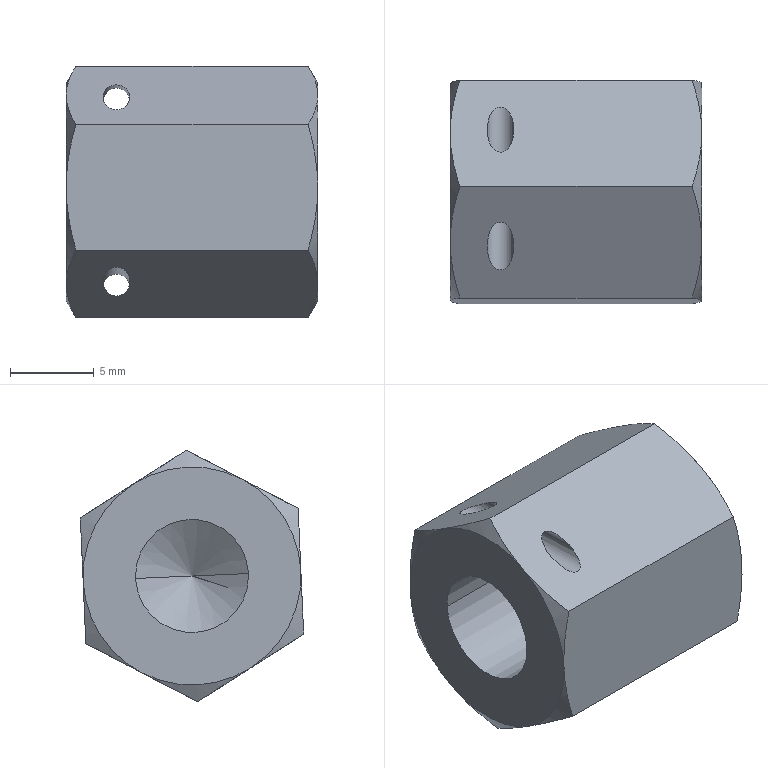Part | SolidWorks | features BaseBody 1 | 1 solid | 32 faces | box 15 x 13.316 x 14.997 mm | volume 1682 mm3 | cone 14 | plane 10 | cylinder 8 | commonest cylinder face diameters 1.6 x4 6.75 x2 8.5 x2
STEP:
#1=CARTESIAN_POINT('',(447.8,161.77,5.647));
#2=VERTEX_POINT('',#1);
#3=CARTESIAN_POINT('',(449.4,161.77,5.647));
#4=VERTEX_POINT('',#3);
#5=CARTESIAN_POINT('',(447.8,161.77,5.647));
#6=CARTESIAN_POINT('',(447.8,164.609,7.124));
#7=CARTESIAN_POINT('',(449.4,164.609,7.124));
#8=CARTESIAN_POINT('',(449.4,161.77,5.647));
#9=(BOUNDED_CURVE()B_SPLINE_CURVE(3,(#5,#6,#7,#8),.UNSPECIFIED.,.F.,.T.)B_SPLINE_CURVE_WITH_KNOTS((4,4),(4.712,7.854),.UNSPECIFIED.)CURVE()GEOMETRIC_REPRESENTATION_ITEM()RATIONAL_B_SPLINE_CURVE((1.,0.3333,0.3333,1.))REPRESENTATION_ITEM(''));
#10=EDGE_CURVE('',#2,#4,#9,.T.);
#11=ORIENTED_EDGE('',*,*,#10,.F.);
#12=CARTESIAN_POINT('',(447.8,168.711,5.343));
#13=VERTEX_POINT('',#12);
#14=CARTESIAN_POINT('',(447.8,158.747,5.779));
#15=DIRECTION('',(0.,0.999,-0.04373));
#16=VECTOR('',#15,1000.);
#17=LINE('',#14,#16);
#18=EDGE_CURVE('',#2,#13,#17,.T.);
#19=ORIENTED_EDGE('',*,*,#18,.T.);
#20=CARTESIAN_POINT('',(449.4,168.711,5.343));
#21=VERTEX_POINT('',#20);
#22=CARTESIAN_POINT('',(449.4,168.711,5.343));
#23=CARTESIAN_POINT('',(449.4,166.012,7.062));
#24=CARTESIAN_POINT('',(447.8,166.012,7.062));
#25=CARTESIAN_POINT('',(447.8,168.711,5.343));
#26=(BOUNDED_CURVE()B_SPLINE_CURVE(3,(#22,#23,#24,#25),.UNSPECIFIED.,.F.,.T.)B_SPLINE_CURVE_WITH_KNOTS((4,4),(1.571,4.712),.UNSPECIFIED.)CURVE()GEOMETRIC_REPRESENTATION_ITEM()RATIONAL_B_SPLINE_CURVE((1.,0.3333,0.3333,1.))REPRESENTATION_ITEM(''));
#27=EDGE_CURVE('',#21,#13,#26,.T.);
#28=ORIENTED_EDGE('',*,*,#27,.F.);
#29=CARTESIAN_POINT('',(449.4,158.747,5.779));
#30=DIRECTION('',(0.,0.999,-0.04373));
#31=VECTOR('',#30,1000.);
#32=LINE('',#29,#31);
#33=EDGE_CURVE('',#4,#21,#32,.T.);
#34=ORIENTED_EDGE('',*,*,#33,.F.);
#35=EDGE_LOOP('',(#11,#19,#28,#34));
#36=FACE_OUTER_BOUND('',#35,.T.);
#37=CARTESIAN_POINT('',(448.6,158.747,5.779));
#38=DIRECTION('',(0.,0.999,-0.04373));
#39=DIRECTION('',(1.,0.,0.));
#40=AXIS2_PLACEMENT_3D('',#37,#38,#39);
#41=CYLINDRICAL_SURFACE('',#40,0.8);
#42=ADVANCED_FACE('',(#36),#41,.F.);
#43=CARTESIAN_POINT('',(447.8,161.289,-5.343));
#44=VERTEX_POINT('',#43);
#45=CARTESIAN_POINT('',(449.4,161.289,-5.343));
#46=VERTEX_POINT('',#45);
#47=CARTESIAN_POINT('',(447.8,161.289,-5.343));
#48=CARTESIAN_POINT('',(447.8,158.59,-3.623));
#49=CARTESIAN_POINT('',(449.4,158.59,-3.623));
#50=CARTESIAN_POINT('',(449.4,161.289,-5.343));
#51=(BOUNDED_CURVE()B_SPLINE_CURVE(3,(#47,#48,#49,#50),.UNSPECIFIED.,.F.,.T.)B_SPLINE_CURVE_WITH_KNOTS((4,4),(1.571,4.712),.UNSPECIFIED.)CURVE()GEOMETRIC_REPRESENTATION_ITEM()RATIONAL_B_SPLINE_CURVE((1.,0.3333,0.3333,1.))REPRESENTATION_ITEM(''));
#52=EDGE_CURVE('',#44,#46,#51,.T.);
#53=ORIENTED_EDGE('',*,*,#52,.F.);
#54=CARTESIAN_POINT('',(447.8,168.23,-5.647));
#55=VERTEX_POINT('',#54);
#56=CARTESIAN_POINT('',(447.8,158.266,-5.211));
#57=DIRECTION('',(0.,0.999,-0.04373));
#58=VECTOR('',#57,1000.);
#59=LINE('',#56,#58);
#60=EDGE_CURVE('',#44,#55,#59,.T.);
#61=ORIENTED_EDGE('',*,*,#60,.T.);
#62=CARTESIAN_POINT('',(449.4,168.23,-5.647));
#63=VERTEX_POINT('',#62);
#64=CARTESIAN_POINT('',(449.4,168.23,-5.647));
#65=CARTESIAN_POINT('',(449.4,171.068,-4.169));
#66=CARTESIAN_POINT('',(447.8,171.068,-4.169));
#67=CARTESIAN_POINT('',(447.8,168.23,-5.647));
#68=(BOUNDED_CURVE()B_SPLINE_CURVE(3,(#64,#65,#66,#67),.UNSPECIFIED.,.F.,.T.)B_SPLINE_CURVE_WITH_KNOTS((4,4),(4.712,7.854),.UNSPECIFIED.)CURVE()GEOMETRIC_REPRESENTATION_ITEM()RATIONAL_B_SPLINE_CURVE((1.,0.3333,0.3333,1.))REPRESENTATION_ITEM(''));
#69=EDGE_CURVE('',#63,#55,#68,.T.);
#70=ORIENTED_EDGE('',*,*,#69,.F.);
#71=CARTESIAN_POINT('',(449.4,158.266,-5.211));
#72=DIRECTION('',(0.,0.999,-0.04373));
#73=VECTOR('',#72,1000.);
#74=LINE('',#71,#73);
#75=EDGE_CURVE('',#46,#63,#74,.T.);
#76=ORIENTED_EDGE('',*,*,#75,.F.);
#77=EDGE_LOOP('',(#53,#61,#70,#76));
#78=FACE_OUTER_BOUND('',#77,.T.);
#79=CARTESIAN_POINT('',(448.6,158.266,-5.211));
#80=DIRECTION('',(0.,0.999,-0.04373));
#81=DIRECTION('',(1.,0.,0.));
#82=AXIS2_PLACEMENT_3D('',#79,#80,#81);
#83=CYLINDRICAL_SURFACE('',#82,0.8);
#84=ADVANCED_FACE('',(#78),#83,.F.);
#85=CARTESIAN_POINT('',(458.628,165.,0.));
#86=VERTEX_POINT('',#85);
#87=CARTESIAN_POINT('',(456.6,168.372,-0.1476));
#88=VERTEX_POINT('',#87);
#89=CARTESIAN_POINT('',(456.6,168.372,-0.1476));
#90=DIRECTION('',(-0.515,0.8563,-0.03748));
#91=VECTOR('',#90,1000.);
#92=LINE('',#89,#91);
#93=EDGE_CURVE('',#86,#88,#92,.T.);
#94=ORIENTED_EDGE('',*,*,#93,.F.);
#95=CARTESIAN_POINT('',(456.6,161.628,0.1476));
#96=VERTEX_POINT('',#95);
#97=CARTESIAN_POINT('',(456.6,161.628,0.1476));
#98=DIRECTION('',(-0.515,-0.8563,0.03748));
#99=VECTOR('',#98,1000.);
#100=LINE('',#97,#99);
#101=EDGE_CURVE('',#86,#96,#100,.T.);
#102=ORIENTED_EDGE('',*,*,#101,.T.);
#103=CARTESIAN_POINT('',(456.6,165.,0.));
#104=DIRECTION('',(1.,0.,0.));
#105=DIRECTION('',(0.,0.999,-0.04373));
#106=AXIS2_PLACEMENT_3D('',#103,#104,#105);
#107=CIRCLE('',#106,3.375);
#108=EDGE_CURVE('',#88,#96,#107,.T.);
#109=ORIENTED_EDGE('',*,*,#108,.F.);
#110=EDGE_LOOP('',(#94,#102,#109));
#111=FACE_OUTER_BOUND('',#110,.T.);
#112=CARTESIAN_POINT('',(456.6,165.,0.));
#113=DIRECTION('',(-1.,0.,0.));
#114=DIRECTION('',(0.,0.999,-0.04373));
#115=AXIS2_PLACEMENT_3D('',#112,#113,#114);
#116=CONICAL_SURFACE('',#115,3.375,1.03);
#117=ADVANCED_FACE('',(#111),#116,.F.);
#118=CARTESIAN_POINT('',(456.6,160.754,0.1858));
#119=VERTEX_POINT('',#118);
#120=CARTESIAN_POINT('',(456.6,169.246,-0.1858));
#121=VERTEX_POINT('',#120);
#122=CARTESIAN_POINT('',(456.6,165.,0.));
#123=DIRECTION('',(-1.,0.,0.));
#124=DIRECTION('',(0.,0.999,-0.04373));
#125=AXIS2_PLACEMENT_3D('',#122,#123,#124);
#126=CIRCLE('',#125,4.25);
#127=EDGE_CURVE('',#119,#121,#126,.T.);
#128=ORIENTED_EDGE('',*,*,#127,.F.);
#129=CARTESIAN_POINT('',(453.6,160.754,0.1858));
#130=VERTEX_POINT('',#129);
#131=CARTESIAN_POINT('',(456.6,160.754,0.1858));
#132=DIRECTION('',(-1.,0.,0.));
#133=VECTOR('',#132,1000.);
#134=LINE('',#131,#133);
#135=EDGE_CURVE('',#119,#130,#134,.T.);
#136=ORIENTED_EDGE('',*,*,#135,.T.);
#137=CARTESIAN_POINT('',(453.6,169.246,-0.1858));
#138=VERTEX_POINT('',#137);
#139=CARTESIAN_POINT('',(453.6,165.,0.));
#140=DIRECTION('',(-1.,0.,0.));
#141=DIRECTION('',(0.,0.999,-0.04373));
#142=AXIS2_PLACEMENT_3D('',#139,#140,#141);
#143=CIRCLE('',#142,4.25);
#144=EDGE_CURVE('',#130,#138,#143,.T.);
#145=ORIENTED_EDGE('',*,*,#144,.T.);
#146=CARTESIAN_POINT('',(456.6,169.246,-0.1858));
#147=DIRECTION('',(-1.,0.,0.));
#148=VECTOR('',#147,1000.);
#149=LINE('',#146,#148);
#150=EDGE_CURVE('',#121,#138,#149,.T.);
#151=ORIENTED_EDGE('',*,*,#150,.F.);
#152=EDGE_LOOP('',(#128,#136,#145,#151));
#153=FACE_OUTER_BOUND('',#152,.T.);
#154=CARTESIAN_POINT('',(456.6,165.,0.));
#155=DIRECTION('',(-1.,0.,0.));
#156=DIRECTION('',(0.,0.999,-0.04373));
#157=AXIS2_PLACEMENT_3D('',#154,#155,#156);
#158=CYLINDRICAL_SURFACE('',#157,4.25);
#159=ADVANCED_FACE('',(#153),#158,.F.);
#160=CARTESIAN_POINT('',(453.6,168.372,-0.1476));
#161=VERTEX_POINT('',#160);
#162=CARTESIAN_POINT('',(453.6,161.628,0.1476));
#163=VERTEX_POINT('',#162);
#164=CARTESIAN_POINT('',(453.6,165.,0.));
#165=DIRECTION('',(1.,0.,0.));
#166=DIRECTION('',(0.,0.999,-0.04373));
#167=AXIS2_PLACEMENT_3D('',#164,#165,#166);
#168=CIRCLE('',#167,3.375);
#169=EDGE_CURVE('',#161,#163,#168,.T.);
#170=ORIENTED_EDGE('',*,*,#169,.T.);
#171=CARTESIAN_POINT('',(445.6,161.628,0.1476));
#172=VERTEX_POINT('',#171);
#173=CARTESIAN_POINT('',(456.6,161.628,0.1476));
#174=DIRECTION('',(-1.,0.,0.));
#175=VECTOR('',#174,1000.);
#176=LINE('',#173,#175);
#177=EDGE_CURVE('',#163,#172,#176,.T.);
#178=ORIENTED_EDGE('',*,*,#177,.T.);
#179=CARTESIAN_POINT('',(445.6,168.372,-0.1476));
#180=VERTEX_POINT('',#179);
#181=CARTESIAN_POINT('',(445.6,165.,0.));
#182=DIRECTION('',(-1.,0.,0.));
#183=DIRECTION('',(0.,0.999,-0.04373));
#184=AXIS2_PLACEMENT_3D('',#181,#182,#183);
#185=CIRCLE('',#184,3.375);
#186=EDGE_CURVE('',#172,#180,#185,.T.);
#187=ORIENTED_EDGE('',*,*,#186,.T.);
#188=CARTESIAN_POINT('',(456.6,168.372,-0.1476));
#189=DIRECTION('',(-1.,0.,0.));
#190=VECTOR('',#189,1000.);
#191=LINE('',#188,#190);
#192=EDGE_CURVE('',#161,#180,#191,.T.);
#193=ORIENTED_EDGE('',*,*,#192,.F.);
#194=EDGE_LOOP('',(#170,#178,#187,#193));
#195=FACE_OUTER_BOUND('',#194,.T.);
#196=CARTESIAN_POINT('',(456.6,165.,0.));
#197=DIRECTION('',(-1.,0.,0.));
#198=DIRECTION('',(0.,0.999,-0.04373));
#199=AXIS2_PLACEMENT_3D('',#196,#197,#198);
#200=CYLINDRICAL_SURFACE('',#199,3.375);
#201=ADVANCED_FACE('',(#195),#200,.F.);
#202=ORIENTED_EDGE('',*,*,#69,.T.);
#203=CARTESIAN_POINT('',(447.8,168.23,-5.647));
#204=CARTESIAN_POINT('',(447.8,165.391,-7.124));
#205=CARTESIAN_POINT('',(449.4,165.391,-7.124));
#206=CARTESIAN_POINT('',(449.4,168.23,-5.647));
#207=(BOUNDED_CURVE()B_SPLINE_CURVE(3,(#203,#204,#205,#206),.UNSPECIFIED.,.F.,.T.)B_SPLINE_CURVE_WITH_KNOTS((4,4),(1.571,4.712),.UNSPECIFIED.)CURVE()GEOMETRIC_REPRESENTATION_ITEM()RATIONAL_B_SPLINE_CURVE((1.,0.3333,0.3333,1.))REPRESENTATION_ITEM(''));
#208=EDGE_CURVE('',#55,#63,#207,.T.);
#209=ORIENTED_EDGE('',*,*,#208,.T.);
#210=EDGE_LOOP('',(#202,#209));
#211=FACE_BOUND('',#210,.T.);
#212=CARTESIAN_POINT('',(460.019,164.672,-7.498));
#213=VERTEX_POINT('',#212);
#214=CARTESIAN_POINT('',(460.6,168.001,-5.766));
#215=VERTEX_POINT('',#214);
#216=CARTESIAN_POINT('',(460.019,164.672,-7.498));
#217=CARTESIAN_POINT('',(460.197,165.216,-7.215));
#218=CARTESIAN_POINT('',(460.343,165.765,-6.929));
#219=CARTESIAN_POINT('',(460.545,166.873,-6.353));
#220=CARTESIAN_POINT('',(460.6,167.434,-6.061));
#221=CARTESIAN_POINT('',(460.6,168.001,-5.766));
#222=B_SPLINE_CURVE_WITH_KNOTS('',3,(#216,#217,#218,#219,#220,#221),.UNSPECIFIED.,.F.,.F.,(4,2,4),(0.000000238,0.001899,0.003797),.UNSPECIFIED.);
#223=EDGE_CURVE('',#213,#215,#222,.T.);
#224=ORIENTED_EDGE('',*,*,#223,.F.);
#225=CARTESIAN_POINT('',(446.181,164.672,-7.498));
#226=VERTEX_POINT('',#225);
#227=CARTESIAN_POINT('',(445.6,164.672,-7.498));
#228=DIRECTION('',(1.,0.,0.));
#229=VECTOR('',#228,1000.);
#230=LINE('',#227,#229);
#231=EDGE_CURVE('',#226,#213,#230,.T.);
#232=ORIENTED_EDGE('',*,*,#231,.F.);
#233=CARTESIAN_POINT('',(445.6,168.001,-5.766));
#234=VERTEX_POINT('',#233);
#235=CARTESIAN_POINT('',(445.6,168.001,-5.766));
#236=CARTESIAN_POINT('',(445.6,167.718,-5.913));
#237=CARTESIAN_POINT('',(445.614,167.434,-6.061));
#238=CARTESIAN_POINT('',(445.667,166.873,-6.353));
#239=CARTESIAN_POINT('',(445.706,166.594,-6.498));
#240=CARTESIAN_POINT('',(445.858,165.763,-6.931));
#241=CARTESIAN_POINT('',(446.004,165.215,-7.216));
#242=CARTESIAN_POINT('',(446.181,164.672,-7.498));
#243=B_SPLINE_CURVE_WITH_KNOTS('',3,(#235,#236,#237,#238,#239,#240,#241,#242),.UNSPECIFIED.,.F.,.F.,(4,2,2,4),(0.003797,0.004743,0.005689,0.00758),.UNSPECIFIED.);
#244=EDGE_CURVE('',#234,#226,#243,.T.);
#245=ORIENTED_EDGE('',*,*,#244,.F.);
#246=CARTESIAN_POINT('',(446.181,171.33,-4.033));
#247=VERTEX_POINT('',#246);
#248=CARTESIAN_POINT('',(446.181,171.33,-4.033));
#249=CARTESIAN_POINT('',(446.003,170.785,-4.317));
#250=CARTESIAN_POINT('',(445.857,170.237,-4.602));
#251=CARTESIAN_POINT('',(445.655,169.128,-5.179));
#252=CARTESIAN_POINT('',(445.6,168.568,-5.471));
#253=CARTESIAN_POINT('',(445.6,168.001,-5.766));
#254=B_SPLINE_CURVE_WITH_KNOTS('',3,(#248,#249,#250,#251,#252,#253),.UNSPECIFIED.,.F.,.F.,(4,2,4),(0.000000238,0.001899,0.003797),.UNSPECIFIED.);
#255=EDGE_CURVE('',#247,#234,#254,.T.);
#256=ORIENTED_EDGE('',*,*,#255,.F.);
#257=CARTESIAN_POINT('',(460.019,171.33,-4.033));
#258=VERTEX_POINT('',#257);
#259=CARTESIAN_POINT('',(445.6,171.33,-4.033));
#260=DIRECTION('',(1.,0.,0.));
#261=VECTOR('',#260,1000.);
#262=LINE('',#259,#261);
#263=EDGE_CURVE('',#247,#258,#262,.T.);
#264=ORIENTED_EDGE('',*,*,#263,.T.);
#265=CARTESIAN_POINT('',(460.6,168.001,-5.766));
#266=CARTESIAN_POINT('',(460.6,168.283,-5.619));
#267=CARTESIAN_POINT('',(460.586,168.567,-5.471));
#268=CARTESIAN_POINT('',(460.533,169.128,-5.179));
#269=CARTESIAN_POINT('',(460.494,169.407,-5.034));
#270=CARTESIAN_POINT('',(460.342,170.239,-4.601));
#271=CARTESIAN_POINT('',(460.196,170.786,-4.316));
#272=CARTESIAN_POINT('',(460.019,171.33,-4.033));
#273=B_SPLINE_CURVE_WITH_KNOTS('',3,(#265,#266,#267,#268,#269,#270,#271,#272),.UNSPECIFIED.,.F.,.F.,(4,2,2,4),(0.003797,0.004743,0.005689,0.00758),.UNSPECIFIED.);
#274=EDGE_CURVE('',#215,#258,#273,.T.);
#275=ORIENTED_EDGE('',*,*,#274,.F.);
#276=EDGE_LOOP('',(#224,#232,#245,#256,#264,#275));
#277=FACE_OUTER_BOUND('',#276,.T.);
#278=CARTESIAN_POINT('',(445.6,171.33,-4.033));
#279=DIRECTION('',(0.,-0.4617,0.8871));
#280=DIRECTION('',(0.,0.8871,0.4617));
#281=AXIS2_PLACEMENT_3D('',#278,#279,#280);
#282=PLANE('',#281);
#283=ADVANCED_FACE('',(#211,#277),#282,.F.);
#284=CARTESIAN_POINT('',(449.4,161.289,-5.343));
#285=CARTESIAN_POINT('',(449.4,163.988,-7.062));
#286=CARTESIAN_POINT('',(447.8,163.988,-7.062));
#287=CARTESIAN_POINT('',(447.8,161.289,-5.343));
#288=(BOUNDED_CURVE()B_SPLINE_CURVE(3,(#284,#285,#286,#287),.UNSPECIFIED.,.F.,.T.)B_SPLINE_CURVE_WITH_KNOTS((4,4),(4.712,7.854),.UNSPECIFIED.)CURVE()GEOMETRIC_REPRESENTATION_ITEM()RATIONAL_B_SPLINE_CURVE((1.,0.3333,0.3333,1.))REPRESENTATION_ITEM(''));
#289=EDGE_CURVE('',#46,#44,#288,.T.);
#290=ORIENTED_EDGE('',*,*,#289,.T.);
#291=ORIENTED_EDGE('',*,*,#52,.T.);
#292=EDGE_LOOP('',(#290,#291));
#293=FACE_BOUND('',#292,.T.);
#294=CARTESIAN_POINT('',(460.019,158.342,-3.465));
#295=VERTEX_POINT('',#294);
#296=CARTESIAN_POINT('',(460.6,161.507,-5.482));
#297=VERTEX_POINT('',#296);
#298=CARTESIAN_POINT('',(460.019,158.342,-3.465));
#299=CARTESIAN_POINT('',(460.197,158.86,-3.795));
#300=CARTESIAN_POINT('',(460.343,159.381,-4.127));
#301=CARTESIAN_POINT('',(460.545,160.435,-4.799));
#302=CARTESIAN_POINT('',(460.6,160.968,-5.138));
#303=CARTESIAN_POINT('',(460.6,161.507,-5.482));
#304=B_SPLINE_CURVE_WITH_KNOTS('',3,(#298,#299,#300,#301,#302,#303),.UNSPECIFIED.,.F.,.F.,(4,2,4),(0.000000238,0.001899,0.003797),.UNSPECIFIED.);
#305=EDGE_CURVE('',#295,#297,#304,.T.);
#306=ORIENTED_EDGE('',*,*,#305,.F.);
#307=CARTESIAN_POINT('',(446.181,158.342,-3.465));
#308=VERTEX_POINT('',#307);
#309=CARTESIAN_POINT('',(445.6,158.342,-3.465));
#310=DIRECTION('',(1.,0.,0.));
#311=VECTOR('',#310,1000.);
#312=LINE('',#309,#311);
#313=EDGE_CURVE('',#308,#295,#312,.T.);
#314=ORIENTED_EDGE('',*,*,#313,.F.);
#315=CARTESIAN_POINT('',(445.6,161.507,-5.482));
#316=VERTEX_POINT('',#315);
#317=CARTESIAN_POINT('',(445.6,161.507,-5.482));
#318=CARTESIAN_POINT('',(445.6,161.238,-5.311));
#319=CARTESIAN_POINT('',(445.614,160.969,-5.139));
#320=CARTESIAN_POINT('',(445.667,160.435,-4.799));
#321=CARTESIAN_POINT('',(445.706,160.17,-4.63));
#322=CARTESIAN_POINT('',(445.858,159.379,-4.126));
#323=CARTESIAN_POINT('',(446.004,158.859,-3.794));
#324=CARTESIAN_POINT('',(446.181,158.342,-3.465));
#325=B_SPLINE_CURVE_WITH_KNOTS('',3,(#317,#318,#319,#320,#321,#322,#323,#324),.UNSPECIFIED.,.F.,.F.,(4,2,2,4),(0.003797,0.004743,0.005689,0.00758),.UNSPECIFIED.);
#326=EDGE_CURVE('',#316,#308,#325,.T.);
#327=ORIENTED_EDGE('',*,*,#326,.F.);
#328=CARTESIAN_POINT('',(446.181,164.672,-7.498));
#329=CARTESIAN_POINT('',(446.003,164.154,-7.168));
#330=CARTESIAN_POINT('',(445.857,163.633,-6.836));
#331=CARTESIAN_POINT('',(445.655,162.579,-6.165));
#332=CARTESIAN_POINT('',(445.6,162.046,-5.825));
#333=CARTESIAN_POINT('',(445.6,161.507,-5.482));
#334=B_SPLINE_CURVE_WITH_KNOTS('',3,(#328,#329,#330,#331,#332,#333),.UNSPECIFIED.,.F.,.F.,(4,2,4),(0.000000238,0.001899,0.003797),.UNSPECIFIED.);
#335=EDGE_CURVE('',#226,#316,#334,.T.);
#336=ORIENTED_EDGE('',*,*,#335,.F.);
#337=ORIENTED_EDGE('',*,*,#231,.T.);
#338=CARTESIAN_POINT('',(460.6,161.507,-5.482));
#339=CARTESIAN_POINT('',(460.6,161.776,-5.653));
#340=CARTESIAN_POINT('',(460.586,162.045,-5.825));
#341=CARTESIAN_POINT('',(460.533,162.579,-6.165));
#342=CARTESIAN_POINT('',(460.494,162.844,-6.334));
#343=CARTESIAN_POINT('',(460.342,163.635,-6.837));
#344=CARTESIAN_POINT('',(460.196,164.155,-7.169));
#345=CARTESIAN_POINT('',(460.019,164.672,-7.498));
#346=B_SPLINE_CURVE_WITH_KNOTS('',3,(#338,#339,#340,#341,#342,#343,#344,#345),.UNSPECIFIED.,.F.,.F.,(4,2,2,4),(0.003797,0.004743,0.005689,0.00758),.UNSPECIFIED.);
#347=EDGE_CURVE('',#297,#213,#346,.T.);
#348=ORIENTED_EDGE('',*,*,#347,.F.);
#349=EDGE_LOOP('',(#306,#314,#327,#336,#337,#348));
#350=FACE_OUTER_BOUND('',#349,.T.);
#351=CARTESIAN_POINT('',(445.6,164.672,-7.498));
#352=DIRECTION('',(0.,0.5374,0.8433));
#353=DIRECTION('',(0.,0.8433,-0.5374));
#354=AXIS2_PLACEMENT_3D('',#351,#352,#353);
#355=PLANE('',#354);
#356=ADVANCED_FACE('',(#293,#350),#355,.F.);
#357=CARTESIAN_POINT('',(460.019,158.67,4.033));
#358=VERTEX_POINT('',#357);
#359=CARTESIAN_POINT('',(460.6,158.506,0.2842));
#360=VERTEX_POINT('',#359);
#361=CARTESIAN_POINT('',(460.019,158.67,4.033));
#362=CARTESIAN_POINT('',(460.196,158.644,3.423));
#363=CARTESIAN_POINT('',(460.343,158.616,2.799));
#364=CARTESIAN_POINT('',(460.545,158.562,1.548));
#365=CARTESIAN_POINT('',(460.6,158.534,0.9189));
#366=CARTESIAN_POINT('',(460.6,158.506,0.2842));
#367=B_SPLINE_CURVE_WITH_KNOTS('',3,(#361,#362,#363,#364,#365,#366),.UNSPECIFIED.,.F.,.F.,(4,2,4),(0.007076,0.008976,0.01088),.UNSPECIFIED.);
#368=EDGE_CURVE('',#358,#360,#367,.T.);
#369=ORIENTED_EDGE('',*,*,#368,.F.);
#370=CARTESIAN_POINT('',(446.181,158.67,4.033));
#371=VERTEX_POINT('',#370);
#372=CARTESIAN_POINT('',(445.6,158.67,4.033));
#373=DIRECTION('',(1.,0.,0.));
#374=VECTOR('',#373,1000.);
#375=LINE('',#372,#374);
#376=EDGE_CURVE('',#371,#358,#375,.T.);
#377=ORIENTED_EDGE('',*,*,#376,.F.);
#378=CARTESIAN_POINT('',(445.6,158.506,0.2842));
#379=VERTEX_POINT('',#378);
#380=CARTESIAN_POINT('',(445.6,158.506,0.2842));
#381=CARTESIAN_POINT('',(445.6,158.534,0.9189));
#382=CARTESIAN_POINT('',(445.655,158.562,1.548));
#383=CARTESIAN_POINT('',(445.857,158.616,2.799));
#384=CARTESIAN_POINT('',(446.004,158.644,3.423));
#385=CARTESIAN_POINT('',(446.181,158.67,4.033));
#386=B_SPLINE_CURVE_WITH_KNOTS('',3,(#380,#381,#382,#383,#384,#385),.UNSPECIFIED.,.F.,.F.,(4,2,4),(0.02975,0.03165,0.03354),.UNSPECIFIED.);
#387=EDGE_CURVE('',#379,#371,#386,.T.);
#388=ORIENTED_EDGE('',*,*,#387,.F.);
#389=CARTESIAN_POINT('',(446.181,158.342,-3.465));
#390=CARTESIAN_POINT('',(446.005,158.369,-2.858));
#391=CARTESIAN_POINT('',(445.86,158.396,-2.244));
#392=CARTESIAN_POINT('',(445.707,158.437,-1.306));
#393=CARTESIAN_POINT('',(445.667,158.45,-0.991));
#394=CARTESIAN_POINT('',(445.614,158.478,-0.3534));
#395=CARTESIAN_POINT('',(445.6,158.492,-0.03342));
#396=CARTESIAN_POINT('',(445.6,158.506,0.2842));
#397=B_SPLINE_CURVE_WITH_KNOTS('',3,(#389,#390,#391,#392,#393,#394,#395,#396),.UNSPECIFIED.,.F.,.F.,(4,2,2,4),(0.02595,0.02785,0.0288,0.02975),.UNSPECIFIED.);
#398=EDGE_CURVE('',#308,#379,#397,.T.);
#399=ORIENTED_EDGE('',*,*,#398,.F.);
#400=ORIENTED_EDGE('',*,*,#313,.T.);
#401=CARTESIAN_POINT('',(460.6,158.506,0.2842));
#402=CARTESIAN_POINT('',(460.6,158.492,-0.03342));
#403=CARTESIAN_POINT('',(460.586,158.478,-0.3534));
#404=CARTESIAN_POINT('',(460.533,158.45,-0.991));
#405=CARTESIAN_POINT('',(460.493,158.437,-1.306));
#406=CARTESIAN_POINT('',(460.34,158.396,-2.244));
#407=CARTESIAN_POINT('',(460.195,158.369,-2.858));
#408=CARTESIAN_POINT('',(460.019,158.342,-3.465));
#409=B_SPLINE_CURVE_WITH_KNOTS('',3,(#401,#402,#403,#404,#405,#406,#407,#408),.UNSPECIFIED.,.F.,.F.,(4,2,2,4),(0.01088,0.01183,0.01278,0.01468),.UNSPECIFIED.);
#410=EDGE_CURVE('',#360,#295,#409,.T.);
#411=ORIENTED_EDGE('',*,*,#410,.F.);
#412=EDGE_LOOP('',(#369,#377,#388,#399,#400,#411));
#413=FACE_OUTER_BOUND('',#412,.T.);
#414=CARTESIAN_POINT('',(445.6,158.342,-3.465));
#415=DIRECTION('',(0.,0.999,-0.04373));
#416=DIRECTION('',(0.,-0.04373,-0.999));
#417=AXIS2_PLACEMENT_3D('',#414,#415,#416);
#418=PLANE('',#417);
#419=ADVANCED_FACE('',(#413),#418,.F.);
#420=CARTESIAN_POINT('',(449.4,161.77,5.647));
#421=CARTESIAN_POINT('',(449.4,158.932,4.169));
#422=CARTESIAN_POINT('',(447.8,158.932,4.169));
#423=CARTESIAN_POINT('',(447.8,161.77,5.647));
#424=(BOUNDED_CURVE()B_SPLINE_CURVE(3,(#420,#421,#422,#423),.UNSPECIFIED.,.F.,.T.)B_SPLINE_CURVE_WITH_KNOTS((4,4),(1.571,4.712),.UNSPECIFIED.)CURVE()GEOMETRIC_REPRESENTATION_ITEM()RATIONAL_B_SPLINE_CURVE((1.,0.3333,0.3333,1.))REPRESENTATION_ITEM(''));
#425=EDGE_CURVE('',#4,#2,#424,.T.);
#426=ORIENTED_EDGE('',*,*,#425,.T.);
#427=ORIENTED_EDGE('',*,*,#10,.T.);
#428=EDGE_LOOP('',(#426,#427));
#429=FACE_BOUND('',#428,.T.);
#430=CARTESIAN_POINT('',(460.019,165.328,7.498));
#431=VERTEX_POINT('',#430);
#432=CARTESIAN_POINT('',(460.6,161.999,5.766));
#433=VERTEX_POINT('',#432);
#434=CARTESIAN_POINT('',(460.019,165.328,7.498));
#435=CARTESIAN_POINT('',(460.197,164.784,7.215));
#436=CARTESIAN_POINT('',(460.343,164.235,6.929));
#437=CARTESIAN_POINT('',(460.545,163.127,6.353));
#438=CARTESIAN_POINT('',(460.6,162.566,6.061));
#439=CARTESIAN_POINT('',(460.6,161.999,5.766));
#440=B_SPLINE_CURVE_WITH_KNOTS('',3,(#434,#435,#436,#437,#438,#439),.UNSPECIFIED.,.F.,.F.,(4,2,4),(0.000000238,0.001899,0.003797),.UNSPECIFIED.);
#441=EDGE_CURVE('',#431,#433,#440,.T.);
#442=ORIENTED_EDGE('',*,*,#441,.F.);
#443=CARTESIAN_POINT('',(446.181,165.328,7.498));
#444=VERTEX_POINT('',#443);
#445=CARTESIAN_POINT('',(445.6,165.328,7.498));
#446=DIRECTION('',(1.,0.,0.));
#447=VECTOR('',#446,1000.);
#448=LINE('',#445,#447);
#449=EDGE_CURVE('',#444,#431,#448,.T.);
#450=ORIENTED_EDGE('',*,*,#449,.F.);
#451=CARTESIAN_POINT('',(445.6,161.999,5.766));
#452=VERTEX_POINT('',#451);
#453=CARTESIAN_POINT('',(445.6,161.999,5.766));
#454=CARTESIAN_POINT('',(445.6,162.282,5.913));
#455=CARTESIAN_POINT('',(445.614,162.566,6.061));
#456=CARTESIAN_POINT('',(445.667,163.127,6.353));
#457=CARTESIAN_POINT('',(445.706,163.406,6.498));
#458=CARTESIAN_POINT('',(445.858,164.237,6.931));
#459=CARTESIAN_POINT('',(446.004,164.785,7.216));
#460=CARTESIAN_POINT('',(446.181,165.328,7.498));
#461=B_SPLINE_CURVE_WITH_KNOTS('',3,(#453,#454,#455,#456,#457,#458,#459,#460),.UNSPECIFIED.,.F.,.F.,(4,2,2,4),(0.003797,0.004743,0.005689,0.00758),.UNSPECIFIED.);
#462=EDGE_CURVE('',#452,#444,#461,.T.);
#463=ORIENTED_EDGE('',*,*,#462,.F.);
#464=CARTESIAN_POINT('',(446.181,158.67,4.033));
#465=CARTESIAN_POINT('',(446.003,159.215,4.317));
#466=CARTESIAN_POINT('',(445.857,159.763,4.602));
#467=CARTESIAN_POINT('',(445.655,160.872,5.179));
#468=CARTESIAN_POINT('',(445.6,161.432,5.471));
#469=CARTESIAN_POINT('',(445.6,161.999,5.766));
#470=B_SPLINE_CURVE_WITH_KNOTS('',3,(#464,#465,#466,#467,#468,#469),.UNSPECIFIED.,.F.,.F.,(4,2,4),(0.000000238,0.001899,0.003797),.UNSPECIFIED.);
#471=EDGE_CURVE('',#371,#452,#470,.T.);
#472=ORIENTED_EDGE('',*,*,#471,.F.);
#473=ORIENTED_EDGE('',*,*,#376,.T.);
#474=CARTESIAN_POINT('',(460.6,161.999,5.766));
#475=CARTESIAN_POINT('',(460.6,161.717,5.619));
#476=CARTESIAN_POINT('',(460.586,161.433,5.471));
#477=CARTESIAN_POINT('',(460.533,160.872,5.179));
#478=CARTESIAN_POINT('',(460.494,160.593,5.034));
#479=CARTESIAN_POINT('',(460.342,159.761,4.601));
#480=CARTESIAN_POINT('',(460.196,159.214,4.316));
#481=CARTESIAN_POINT('',(460.019,158.67,4.033));
#482=B_SPLINE_CURVE_WITH_KNOTS('',3,(#474,#475,#476,#477,#478,#479,#480,#481),.UNSPECIFIED.,.F.,.F.,(4,2,2,4),(0.003797,0.004743,0.005689,0.00758),.UNSPECIFIED.);
#483=EDGE_CURVE('',#433,#358,#482,.T.);
#484=ORIENTED_EDGE('',*,*,#483,.F.);
#485=EDGE_LOOP('',(#442,#450,#463,#472,#473,#484));
#486=FACE_OUTER_BOUND('',#485,.T.);
#487=CARTESIAN_POINT('',(445.6,158.67,4.033));
#488=DIRECTION('',(0.,0.4617,-0.8871));
#489=DIRECTION('',(0.,-0.8871,-0.4617));
#490=AXIS2_PLACEMENT_3D('',#487,#488,#489);
#491=PLANE('',#490);
#492=ADVANCED_FACE('',(#429,#486),#491,.F.);
#493=ORIENTED_EDGE('',*,*,#27,.T.);
#494=CARTESIAN_POINT('',(447.8,168.711,5.343));
#495=CARTESIAN_POINT('',(447.8,171.41,3.623));
#496=CARTESIAN_POINT('',(449.4,171.41,3.623));
#497=CARTESIAN_POINT('',(449.4,168.711,5.343));
#498=(BOUNDED_CURVE()B_SPLINE_CURVE(3,(#494,#495,#496,#497),.UNSPECIFIED.,.F.,.T.)B_SPLINE_CURVE_WITH_KNOTS((4,4),(4.712,7.854),.UNSPECIFIED.)CURVE()GEOMETRIC_REPRESENTATION_ITEM()RATIONAL_B_SPLINE_CURVE((1.,0.3333,0.3333,1.))REPRESENTATION_ITEM(''));
#499=EDGE_CURVE('',#13,#21,#498,.T.);
#500=ORIENTED_EDGE('',*,*,#499,.T.);
#501=EDGE_LOOP('',(#493,#500));
#502=FACE_BOUND('',#501,.T.);
#503=CARTESIAN_POINT('',(460.019,171.658,3.465));
#504=VERTEX_POINT('',#503);
#505=CARTESIAN_POINT('',(460.6,168.493,5.482));
#506=VERTEX_POINT('',#505);
#507=CARTESIAN_POINT('',(460.019,171.658,3.465));
#508=CARTESIAN_POINT('',(460.197,171.14,3.795));
#509=CARTESIAN_POINT('',(460.343,170.619,4.127));
#510=CARTESIAN_POINT('',(460.545,169.565,4.799));
#511=CARTESIAN_POINT('',(460.6,169.032,5.138));
#512=CARTESIAN_POINT('',(460.6,168.493,5.482));
#513=B_SPLINE_CURVE_WITH_KNOTS('',3,(#507,#508,#509,#510,#511,#512),.UNSPECIFIED.,.F.,.F.,(4,2,4),(0.000000238,0.001899,0.003797),.UNSPECIFIED.);
#514=EDGE_CURVE('',#504,#506,#513,.T.);
#515=ORIENTED_EDGE('',*,*,#514,.F.);
#516=CARTESIAN_POINT('',(446.181,171.658,3.465));
#517=VERTEX_POINT('',#516);
#518=CARTESIAN_POINT('',(445.6,171.658,3.465));
#519=DIRECTION('',(1.,0.,0.));
#520=VECTOR('',#519,1000.);
#521=LINE('',#518,#520);
#522=EDGE_CURVE('',#517,#504,#521,.T.);
#523=ORIENTED_EDGE('',*,*,#522,.F.);
#524=CARTESIAN_POINT('',(445.6,168.493,5.482));
#525=VERTEX_POINT('',#524);
#526=CARTESIAN_POINT('',(445.6,168.493,5.482));
#527=CARTESIAN_POINT('',(445.6,168.762,5.311));
#528=CARTESIAN_POINT('',(445.614,169.031,5.139));
#529=CARTESIAN_POINT('',(445.667,169.565,4.799));
#530=CARTESIAN_POINT('',(445.706,169.83,4.63));
#531=CARTESIAN_POINT('',(445.858,170.621,4.126));
#532=CARTESIAN_POINT('',(446.004,171.141,3.794));
#533=CARTESIAN_POINT('',(446.181,171.658,3.465));
#534=B_SPLINE_CURVE_WITH_KNOTS('',3,(#526,#527,#528,#529,#530,#531,#532,#533),.UNSPECIFIED.,.F.,.F.,(4,2,2,4),(0.003797,0.004743,0.005689,0.00758),.UNSPECIFIED.);
#535=EDGE_CURVE('',#525,#517,#534,.T.);
#536=ORIENTED_EDGE('',*,*,#535,.F.);
#537=CARTESIAN_POINT('',(446.181,165.328,7.498));
#538=CARTESIAN_POINT('',(446.003,165.846,7.168));
#539=CARTESIAN_POINT('',(445.857,166.367,6.836));
#540=CARTESIAN_POINT('',(445.655,167.421,6.165));
#541=CARTESIAN_POINT('',(445.6,167.954,5.825));
#542=CARTESIAN_POINT('',(445.6,168.493,5.482));
#543=B_SPLINE_CURVE_WITH_KNOTS('',3,(#537,#538,#539,#540,#541,#542),.UNSPECIFIED.,.F.,.F.,(4,2,4),(0.000000238,0.001899,0.003797),.UNSPECIFIED.);
#544=EDGE_CURVE('',#444,#525,#543,.T.);
#545=ORIENTED_EDGE('',*,*,#544,.F.);
#546=ORIENTED_EDGE('',*,*,#449,.T.);
#547=CARTESIAN_POINT('',(460.6,168.493,5.482));
#548=CARTESIAN_POINT('',(460.6,168.224,5.653));
#549=CARTESIAN_POINT('',(460.586,167.955,5.825));
#550=CARTESIAN_POINT('',(460.533,167.421,6.165));
#551=CARTESIAN_POINT('',(460.494,167.156,6.334));
#552=CARTESIAN_POINT('',(460.342,166.365,6.837));
#553=CARTESIAN_POINT('',(460.196,165.845,7.169));
#554=CARTESIAN_POINT('',(460.019,165.328,7.498));
#555=B_SPLINE_CURVE_WITH_KNOTS('',3,(#547,#548,#549,#550,#551,#552,#553,#554),.UNSPECIFIED.,.F.,.F.,(4,2,2,4),(0.003797,0.004743,0.005689,0.00758),.UNSPECIFIED.);
#556=EDGE_CURVE('',#506,#431,#555,.T.);
#557=ORIENTED_EDGE('',*,*,#556,.F.);
#558=EDGE_LOOP('',(#515,#523,#536,#545,#546,#557));
#559=FACE_OUTER_BOUND('',#558,.T.);
#560=CARTESIAN_POINT('',(445.6,165.328,7.498));
#561=DIRECTION('',(0.,-0.5374,-0.8433));
#562=DIRECTION('',(0.,-0.8433,0.5374));
#563=AXIS2_PLACEMENT_3D('',#560,#561,#562);
#564=PLANE('',#563);
#565=ADVANCED_FACE('',(#502,#559),#564,.F.);
#566=CARTESIAN_POINT('',(460.6,171.494,-0.2842));
#567=VERTEX_POINT('',#566);
#568=CARTESIAN_POINT('',(460.019,171.33,-4.033));
#569=CARTESIAN_POINT('',(460.195,171.356,-3.427));
#570=CARTESIAN_POINT('',(460.34,171.383,-2.813));
#571=CARTESIAN_POINT('',(460.493,171.424,-1.875));
#572=CARTESIAN_POINT('',(460.533,171.438,-1.559));
#573=CARTESIAN_POINT('',(460.586,171.466,-0.9219));
#574=CARTESIAN_POINT('',(460.6,171.48,-0.6019));
#575=CARTESIAN_POINT('',(460.6,171.494,-0.2842));
#576=B_SPLINE_CURVE_WITH_KNOTS('',3,(#568,#569,#570,#571,#572,#573,#574,#575),.UNSPECIFIED.,.F.,.F.,(4,2,2,4),(0.02595,0.02785,0.0288,0.02975),.UNSPECIFIED.);
#577=EDGE_CURVE('',#258,#567,#576,.T.);
#578=ORIENTED_EDGE('',*,*,#577,.F.);
#579=ORIENTED_EDGE('',*,*,#263,.F.);
#580=CARTESIAN_POINT('',(445.6,171.494,-0.2842));
#581=VERTEX_POINT('',#580);
#582=CARTESIAN_POINT('',(445.6,171.494,-0.2842));
#583=CARTESIAN_POINT('',(445.6,171.48,-0.6019));
#584=CARTESIAN_POINT('',(445.614,171.466,-0.9219));
#585=CARTESIAN_POINT('',(445.667,171.438,-1.559));
#586=CARTESIAN_POINT('',(445.707,171.424,-1.875));
#587=CARTESIAN_POINT('',(445.86,171.383,-2.813));
#588=CARTESIAN_POINT('',(446.005,171.356,-3.427));
#589=CARTESIAN_POINT('',(446.181,171.33,-4.033));
#590=B_SPLINE_CURVE_WITH_KNOTS('',3,(#582,#583,#584,#585,#586,#587,#588,#589),.UNSPECIFIED.,.F.,.F.,(4,2,2,4),(0.01088,0.01183,0.01278,0.01468),.UNSPECIFIED.);
#591=EDGE_CURVE('',#581,#247,#590,.T.);
#592=ORIENTED_EDGE('',*,*,#591,.F.);
#593=CARTESIAN_POINT('',(446.181,171.658,3.465));
#594=CARTESIAN_POINT('',(446.004,171.631,2.854));
#595=CARTESIAN_POINT('',(445.857,171.604,2.23));
#596=CARTESIAN_POINT('',(445.655,171.549,0.9801));
#597=CARTESIAN_POINT('',(445.6,171.522,0.3505));
#598=CARTESIAN_POINT('',(445.6,171.494,-0.2842));
#599=B_SPLINE_CURVE_WITH_KNOTS('',3,(#593,#594,#595,#596,#597,#598),.UNSPECIFIED.,.F.,.F.,(4,2,4),(0.007076,0.008976,0.01088),.UNSPECIFIED.);
#600=EDGE_CURVE('',#517,#581,#599,.T.);
#601=ORIENTED_EDGE('',*,*,#600,.F.);
#602=ORIENTED_EDGE('',*,*,#522,.T.);
#603=CARTESIAN_POINT('',(460.6,171.494,-0.2842));
#604=CARTESIAN_POINT('',(460.6,171.522,0.3505));
#605=CARTESIAN_POINT('',(460.545,171.549,0.9801));
#606=CARTESIAN_POINT('',(460.343,171.604,2.23));
#607=CARTESIAN_POINT('',(460.196,171.631,2.854));
#608=CARTESIAN_POINT('',(460.019,171.658,3.465));
#609=B_SPLINE_CURVE_WITH_KNOTS('',3,(#603,#604,#605,#606,#607,#608),.UNSPECIFIED.,.F.,.F.,(4,2,4),(0.02975,0.03165,0.03354),.UNSPECIFIED.);
#610=EDGE_CURVE('',#567,#504,#609,.T.);
#611=ORIENTED_EDGE('',*,*,#610,.F.);
#612=EDGE_LOOP('',(#578,#579,#592,#601,#602,#611));
#613=FACE_OUTER_BOUND('',#612,.T.);
#614=CARTESIAN_POINT('',(445.6,171.658,3.465));
#615=DIRECTION('',(0.,-0.999,0.04373));
#616=DIRECTION('',(0.,0.04373,0.999));
#617=AXIS2_PLACEMENT_3D('',#614,#615,#616);
#618=PLANE('',#617);
#619=ADVANCED_FACE('',(#613),#618,.F.);
#620=ORIENTED_EDGE('',*,*,#535,.T.);
#621=ORIENTED_EDGE('',*,*,#600,.T.);
#622=CARTESIAN_POINT('',(445.6,165.,0.));
#623=DIRECTION('',(-1.,0.,0.));
#624=DIRECTION('',(0.,0.999,-0.04373));
#625=AXIS2_PLACEMENT_3D('',#622,#623,#624);
#626=CIRCLE('',#625,6.5);
#627=EDGE_CURVE('',#525,#581,#626,.T.);
#628=ORIENTED_EDGE('',*,*,#627,.F.);
#629=EDGE_LOOP('',(#620,#621,#628));
#630=FACE_OUTER_BOUND('',#629,.T.);
#631=CARTESIAN_POINT('',(445.6,165.,0.));
#632=DIRECTION('',(1.,0.,0.));
#633=DIRECTION('',(0.,0.999,-0.04373));
#634=AXIS2_PLACEMENT_3D('',#631,#632,#633);
#635=CONICAL_SURFACE('',#634,6.5,1.047);
#636=ADVANCED_FACE('',(#630),#635,.T.);
#637=ORIENTED_EDGE('',*,*,#462,.T.);
#638=ORIENTED_EDGE('',*,*,#544,.T.);
#639=CARTESIAN_POINT('',(445.6,165.,0.));
#640=DIRECTION('',(-1.,0.,0.));
#641=DIRECTION('',(0.,0.999,-0.04373));
#642=AXIS2_PLACEMENT_3D('',#639,#640,#641);
#643=CIRCLE('',#642,6.5);
#644=EDGE_CURVE('',#452,#525,#643,.T.);
#645=ORIENTED_EDGE('',*,*,#644,.F.);
#646=EDGE_LOOP('',(#637,#638,#645));
#647=FACE_OUTER_BOUND('',#646,.T.);
#648=CARTESIAN_POINT('',(445.6,165.,0.));
#649=DIRECTION('',(1.,0.,0.));
#650=DIRECTION('',(0.,0.999,-0.04373));
#651=AXIS2_PLACEMENT_3D('',#648,#649,#650);
#652=CONICAL_SURFACE('',#651,6.5,1.047);
#653=ADVANCED_FACE('',(#647),#652,.T.);
#654=ORIENTED_EDGE('',*,*,#387,.T.);
#655=ORIENTED_EDGE('',*,*,#471,.T.);
#656=CARTESIAN_POINT('',(445.6,165.,0.));
#657=DIRECTION('',(-1.,0.,0.));
#658=DIRECTION('',(0.,0.999,-0.04373));
#659=AXIS2_PLACEMENT_3D('',#656,#657,#658);
#660=CIRCLE('',#659,6.5);
#661=EDGE_CURVE('',#379,#452,#660,.T.);
#662=ORIENTED_EDGE('',*,*,#661,.F.);
#663=EDGE_LOOP('',(#654,#655,#662));
#664=FACE_OUTER_BOUND('',#663,.T.);
#665=CARTESIAN_POINT('',(445.6,165.,0.));
#666=DIRECTION('',(1.,0.,0.));
#667=DIRECTION('',(0.,0.999,-0.04373));
#668=AXIS2_PLACEMENT_3D('',#665,#666,#667);
#669=CONICAL_SURFACE('',#668,6.5,1.047);
#670=ADVANCED_FACE('',(#664),#669,.T.);
#671=ORIENTED_EDGE('',*,*,#326,.T.);
#672=ORIENTED_EDGE('',*,*,#398,.T.);
#673=CARTESIAN_POINT('',(445.6,165.,0.));
#674=DIRECTION('',(-1.,0.,0.));
#675=DIRECTION('',(0.,0.999,-0.04373));
#676=AXIS2_PLACEMENT_3D('',#673,#674,#675);
#677=CIRCLE('',#676,6.5);
#678=EDGE_CURVE('',#316,#379,#677,.T.);
#679=ORIENTED_EDGE('',*,*,#678,.F.);
#680=EDGE_LOOP('',(#671,#672,#679));
#681=FACE_OUTER_BOUND('',#680,.T.);
#682=CARTESIAN_POINT('',(445.6,165.,0.));
#683=DIRECTION('',(1.,0.,0.));
#684=DIRECTION('',(0.,0.999,-0.04373));
#685=AXIS2_PLACEMENT_3D('',#682,#683,#684);
#686=CONICAL_SURFACE('',#685,6.5,1.047);
#687=ADVANCED_FACE('',(#681),#686,.T.);
#688=ORIENTED_EDGE('',*,*,#244,.T.);
#689=ORIENTED_EDGE('',*,*,#335,.T.);
#690=CARTESIAN_POINT('',(445.6,165.,0.));
#691=DIRECTION('',(-1.,0.,0.));
#692=DIRECTION('',(0.,0.999,-0.04373));
#693=AXIS2_PLACEMENT_3D('',#690,#691,#692);
#694=CIRCLE('',#693,6.5);
#695=EDGE_CURVE('',#234,#316,#694,.T.);
#696=ORIENTED_EDGE('',*,*,#695,.F.);
#697=EDGE_LOOP('',(#688,#689,#696));
#698=FACE_OUTER_BOUND('',#697,.T.);
#699=CARTESIAN_POINT('',(445.6,165.,0.));
#700=DIRECTION('',(1.,0.,0.));
#701=DIRECTION('',(0.,0.999,-0.04373));
#702=AXIS2_PLACEMENT_3D('',#699,#700,#701);
#703=CONICAL_SURFACE('',#702,6.5,1.047);
#704=ADVANCED_FACE('',(#698),#703,.T.);
#705=ORIENTED_EDGE('',*,*,#255,.T.);
#706=CARTESIAN_POINT('',(445.6,165.,0.));
#707=DIRECTION('',(-1.,0.,0.));
#708=DIRECTION('',(0.,0.999,-0.04373));
#709=AXIS2_PLACEMENT_3D('',#706,#707,#708);
#710=CIRCLE('',#709,6.5);
#711=EDGE_CURVE('',#581,#234,#710,.T.);
#712=ORIENTED_EDGE('',*,*,#711,.F.);
#713=ORIENTED_EDGE('',*,*,#591,.T.);
#714=EDGE_LOOP('',(#705,#712,#713));
#715=FACE_OUTER_BOUND('',#714,.T.);
#716=CARTESIAN_POINT('',(445.6,165.,0.));
#717=DIRECTION('',(1.,0.,0.));
#718=DIRECTION('',(0.,0.999,-0.04373));
#719=AXIS2_PLACEMENT_3D('',#716,#717,#718);
#720=CONICAL_SURFACE('',#719,6.5,1.047);
#721=ADVANCED_FACE('',(#715),#720,.T.);
#722=CARTESIAN_POINT('',(445.6,165.,0.));
#723=DIRECTION('',(-1.,0.,0.));
#724=DIRECTION('',(0.,0.999,-0.04373));
#725=AXIS2_PLACEMENT_3D('',#722,#723,#724);
#726=CIRCLE('',#725,3.375);
#727=EDGE_CURVE('',#180,#172,#726,.T.);
#728=ORIENTED_EDGE('',*,*,#727,.F.);
#729=ORIENTED_EDGE('',*,*,#186,.F.);
#730=EDGE_LOOP('',(#728,#729));
#731=FACE_BOUND('',#730,.T.);
#732=ORIENTED_EDGE('',*,*,#627,.T.);
#733=ORIENTED_EDGE('',*,*,#711,.T.);
#734=ORIENTED_EDGE('',*,*,#695,.T.);
#735=ORIENTED_EDGE('',*,*,#678,.T.);
#736=ORIENTED_EDGE('',*,*,#661,.T.);
#737=ORIENTED_EDGE('',*,*,#644,.T.);
#738=EDGE_LOOP('',(#732,#733,#734,#735,#736,#737));
#739=FACE_OUTER_BOUND('',#738,.T.);
#740=CARTESIAN_POINT('',(445.6,158.014,-10.963));
#741=DIRECTION('',(-1.,0.,0.));
#742=DIRECTION('',(0.,0.999,-0.04373));
#743=AXIS2_PLACEMENT_3D('',#740,#741,#742);
#744=PLANE('',#743);
#745=ADVANCED_FACE('',(#731,#739),#744,.T.);
#746=ORIENTED_EDGE('',*,*,#514,.T.);
#747=CARTESIAN_POINT('',(460.6,165.,0.));
#748=DIRECTION('',(-1.,0.,0.));
#749=DIRECTION('',(0.,0.999,-0.04373));
#750=AXIS2_PLACEMENT_3D('',#747,#748,#749);
#751=CIRCLE('',#750,6.5);
#752=EDGE_CURVE('',#506,#567,#751,.T.);
#753=ORIENTED_EDGE('',*,*,#752,.T.);
#754=ORIENTED_EDGE('',*,*,#610,.T.);
#755=EDGE_LOOP('',(#746,#753,#754));
#756=FACE_OUTER_BOUND('',#755,.T.);
#757=CARTESIAN_POINT('',(460.6,165.,0.));
#758=DIRECTION('',(-1.,0.,0.));
#759=DIRECTION('',(0.,-0.999,0.04373));
#760=AXIS2_PLACEMENT_3D('',#757,#758,#759);
#761=CONICAL_SURFACE('',#760,6.5,1.047);
#762=ADVANCED_FACE('',(#756),#761,.T.);
#763=ORIENTED_EDGE('',*,*,#441,.T.);
#764=CARTESIAN_POINT('',(460.6,165.,0.));
#765=DIRECTION('',(-1.,0.,0.));
#766=DIRECTION('',(0.,0.999,-0.04373));
#767=AXIS2_PLACEMENT_3D('',#764,#765,#766);
#768=CIRCLE('',#767,6.5);
#769=EDGE_CURVE('',#433,#506,#768,.T.);
#770=ORIENTED_EDGE('',*,*,#769,.T.);
#771=ORIENTED_EDGE('',*,*,#556,.T.);
#772=EDGE_LOOP('',(#763,#770,#771));
#773=FACE_OUTER_BOUND('',#772,.T.);
#774=CARTESIAN_POINT('',(460.6,165.,0.));
#775=DIRECTION('',(-1.,0.,0.));
#776=DIRECTION('',(0.,-0.999,0.04373));
#777=AXIS2_PLACEMENT_3D('',#774,#775,#776);
#778=CONICAL_SURFACE('',#777,6.5,1.047);
#779=ADVANCED_FACE('',(#773),#778,.T.);
#780=ORIENTED_EDGE('',*,*,#368,.T.);
#781=CARTESIAN_POINT('',(460.6,165.,0.));
#782=DIRECTION('',(-1.,0.,0.));
#783=DIRECTION('',(0.,0.999,-0.04373));
#784=AXIS2_PLACEMENT_3D('',#781,#782,#783);
#785=CIRCLE('',#784,6.5);
#786=EDGE_CURVE('',#360,#433,#785,.T.);
#787=ORIENTED_EDGE('',*,*,#786,.T.);
#788=ORIENTED_EDGE('',*,*,#483,.T.);
#789=EDGE_LOOP('',(#780,#787,#788));
#790=FACE_OUTER_BOUND('',#789,.T.);
#791=CARTESIAN_POINT('',(460.6,165.,0.));
#792=DIRECTION('',(-1.,0.,0.));
#793=DIRECTION('',(0.,-0.999,0.04373));
#794=AXIS2_PLACEMENT_3D('',#791,#792,#793);
#795=CONICAL_SURFACE('',#794,6.5,1.047);
#796=ADVANCED_FACE('',(#790),#795,.T.);
#797=ORIENTED_EDGE('',*,*,#410,.T.);
#798=ORIENTED_EDGE('',*,*,#305,.T.);
#799=CARTESIAN_POINT('',(460.6,165.,0.));
#800=DIRECTION('',(1.,0.,0.));
#801=DIRECTION('',(0.,-0.999,0.04373));
#802=AXIS2_PLACEMENT_3D('',#799,#800,#801);
#803=CIRCLE('',#802,6.5);
#804=EDGE_CURVE('',#360,#297,#803,.T.);
#805=ORIENTED_EDGE('',*,*,#804,.F.);
#806=EDGE_LOOP('',(#797,#798,#805));
#807=FACE_OUTER_BOUND('',#806,.T.);
#808=CARTESIAN_POINT('',(460.6,165.,0.));
#809=DIRECTION('',(-1.,0.,0.));
#810=DIRECTION('',(0.,-0.999,0.04373));
#811=AXIS2_PLACEMENT_3D('',#808,#809,#810);
#812=CONICAL_SURFACE('',#811,6.5,1.047);
#813=ADVANCED_FACE('',(#807),#812,.T.);
#814=ORIENTED_EDGE('',*,*,#347,.T.);
#815=ORIENTED_EDGE('',*,*,#223,.T.);
#816=CARTESIAN_POINT('',(460.6,165.,0.));
#817=DIRECTION('',(-1.,0.,0.));
#818=DIRECTION('',(0.,0.999,-0.04373));
#819=AXIS2_PLACEMENT_3D('',#816,#817,#818);
#820=CIRCLE('',#819,6.5);
#821=EDGE_CURVE('',#215,#297,#820,.T.);
#822=ORIENTED_EDGE('',*,*,#821,.T.);
#823=EDGE_LOOP('',(#814,#815,#822));
#824=FACE_OUTER_BOUND('',#823,.T.);
#825=CARTESIAN_POINT('',(460.6,165.,0.));
#826=DIRECTION('',(-1.,0.,0.));
#827=DIRECTION('',(0.,-0.999,0.04373));
#828=AXIS2_PLACEMENT_3D('',#825,#826,#827);
#829=CONICAL_SURFACE('',#828,6.5,1.047);
#830=ADVANCED_FACE('',(#824),#829,.T.);
#831=ORIENTED_EDGE('',*,*,#274,.T.);
#832=ORIENTED_EDGE('',*,*,#577,.T.);
#833=CARTESIAN_POINT('',(460.6,165.,0.));
#834=DIRECTION('',(-1.,0.,0.));
#835=DIRECTION('',(0.,0.999,-0.04373));
#836=AXIS2_PLACEMENT_3D('',#833,#834,#835);
#837=CIRCLE('',#836,6.5);
#838=EDGE_CURVE('',#567,#215,#837,.T.);
#839=ORIENTED_EDGE('',*,*,#838,.T.);
#840=EDGE_LOOP('',(#831,#832,#839));
#841=FACE_OUTER_BOUND('',#840,.T.);
#842=CARTESIAN_POINT('',(460.6,165.,0.));
#843=DIRECTION('',(-1.,0.,0.));
#844=DIRECTION('',(0.,-0.999,0.04373));
#845=AXIS2_PLACEMENT_3D('',#842,#843,#844);
#846=CONICAL_SURFACE('',#845,6.5,1.047);
#847=ADVANCED_FACE('',(#841),#846,.T.);
#848=ORIENTED_EDGE('',*,*,#838,.F.);
#849=ORIENTED_EDGE('',*,*,#752,.F.);
#850=ORIENTED_EDGE('',*,*,#769,.F.);
#851=ORIENTED_EDGE('',*,*,#786,.F.);
#852=ORIENTED_EDGE('',*,*,#804,.T.);
#853=ORIENTED_EDGE('',*,*,#821,.F.);
#854=EDGE_LOOP('',(#848,#849,#850,#851,#852,#853));
#855=FACE_OUTER_BOUND('',#854,.T.);
#856=CARTESIAN_POINT('',(460.6,158.014,-10.963));
#857=DIRECTION('',(-1.,0.,0.));
#858=DIRECTION('',(0.,0.999,-0.04373));
#859=AXIS2_PLACEMENT_3D('',#856,#857,#858);
#860=PLANE('',#859);
#861=ADVANCED_FACE('',(#855),#860,.F.);
#862=ORIENTED_EDGE('',*,*,#177,.F.);
#863=CARTESIAN_POINT('',(453.6,165.,0.));
#864=DIRECTION('',(1.,0.,0.));
#865=DIRECTION('',(0.,0.999,-0.04373));
#866=AXIS2_PLACEMENT_3D('',#863,#864,#865);
#867=CIRCLE('',#866,3.375);
#868=EDGE_CURVE('',#163,#161,#867,.T.);
#869=ORIENTED_EDGE('',*,*,#868,.T.);
#870=ORIENTED_EDGE('',*,*,#192,.T.);
#871=ORIENTED_EDGE('',*,*,#727,.T.);
#872=EDGE_LOOP('',(#862,#869,#870,#871));
#873=FACE_OUTER_BOUND('',#872,.T.);
#874=CARTESIAN_POINT('',(456.6,165.,0.));
#875=DIRECTION('',(-1.,0.,0.));
#876=DIRECTION('',(0.,0.999,-0.04373));
#877=AXIS2_PLACEMENT_3D('',#874,#875,#876);
#878=CYLINDRICAL_SURFACE('',#877,3.375);
#879=ADVANCED_FACE('',(#873),#878,.F.);
#880=CARTESIAN_POINT('',(453.6,165.,0.));
#881=DIRECTION('',(-1.,0.,0.));
#882=DIRECTION('',(0.,0.999,-0.04373));
#883=AXIS2_PLACEMENT_3D('',#880,#881,#882);
#884=CIRCLE('',#883,4.25);
#885=EDGE_CURVE('',#138,#130,#884,.T.);
#886=ORIENTED_EDGE('',*,*,#885,.F.);
#887=ORIENTED_EDGE('',*,*,#144,.F.);
#888=EDGE_LOOP('',(#886,#887));
#889=FACE_OUTER_BOUND('',#888,.T.);
#890=ORIENTED_EDGE('',*,*,#169,.F.);
#891=ORIENTED_EDGE('',*,*,#868,.F.);
#892=EDGE_LOOP('',(#890,#891));
#893=FACE_BOUND('',#892,.T.);
#894=CARTESIAN_POINT('',(453.6,165.,0.));
#895=DIRECTION('',(-1.,0.,0.));
#896=DIRECTION('',(0.,0.999,-0.04373));
#897=AXIS2_PLACEMENT_3D('',#894,#895,#896);
#898=PLANE('',#897);
#899=ADVANCED_FACE('',(#889,#893),#898,.F.);
#900=CARTESIAN_POINT('',(456.6,165.,0.));
#901=DIRECTION('',(-1.,0.,0.));
#902=DIRECTION('',(0.,0.999,-0.04373));
#903=AXIS2_PLACEMENT_3D('',#900,#901,#902);
#904=CIRCLE('',#903,4.25);
#905=EDGE_CURVE('',#121,#119,#904,.T.);
#906=ORIENTED_EDGE('',*,*,#905,.T.);
#907=ORIENTED_EDGE('',*,*,#127,.T.);
#908=EDGE_LOOP('',(#906,#907));
#909=FACE_OUTER_BOUND('',#908,.T.);
#910=ORIENTED_EDGE('',*,*,#108,.T.);
#911=CARTESIAN_POINT('',(456.6,165.,0.));
#912=DIRECTION('',(1.,0.,0.));
#913=DIRECTION('',(0.,0.999,-0.04373));
#914=AXIS2_PLACEMENT_3D('',#911,#912,#913);
#915=CIRCLE('',#914,3.375);
#916=EDGE_CURVE('',#96,#88,#915,.T.);
#917=ORIENTED_EDGE('',*,*,#916,.T.);
#918=EDGE_LOOP('',(#910,#917));
#919=FACE_BOUND('',#918,.T.);
#920=CARTESIAN_POINT('',(456.6,165.,0.));
#921=DIRECTION('',(-1.,0.,0.));
#922=DIRECTION('',(0.,0.999,-0.04373));
#923=AXIS2_PLACEMENT_3D('',#920,#921,#922);
#924=PLANE('',#923);
#925=ADVANCED_FACE('',(#909,#919),#924,.T.);
#926=ORIENTED_EDGE('',*,*,#135,.F.);
#927=ORIENTED_EDGE('',*,*,#905,.F.);
#928=ORIENTED_EDGE('',*,*,#150,.T.);
#929=ORIENTED_EDGE('',*,*,#885,.T.);
#930=EDGE_LOOP('',(#926,#927,#928,#929));
#931=FACE_OUTER_BOUND('',#930,.T.);
#932=CARTESIAN_POINT('',(456.6,165.,0.));
#933=DIRECTION('',(-1.,0.,0.));
#934=DIRECTION('',(0.,0.999,-0.04373));
#935=AXIS2_PLACEMENT_3D('',#932,#933,#934);
#936=CYLINDRICAL_SURFACE('',#935,4.25);
#937=ADVANCED_FACE('',(#931),#936,.F.);
#938=ORIENTED_EDGE('',*,*,#101,.F.);
#939=ORIENTED_EDGE('',*,*,#93,.T.);
#940=ORIENTED_EDGE('',*,*,#916,.F.);
#941=EDGE_LOOP('',(#938,#939,#940));
#942=FACE_OUTER_BOUND('',#941,.T.);
#943=CARTESIAN_POINT('',(456.6,165.,0.));
#944=DIRECTION('',(-1.,0.,0.));
#945=DIRECTION('',(0.,0.999,-0.04373));
#946=AXIS2_PLACEMENT_3D('',#943,#944,#945);
#947=CONICAL_SURFACE('',#946,3.375,1.03);
#948=ADVANCED_FACE('',(#942),#947,.F.);
#949=ORIENTED_EDGE('',*,*,#60,.F.);
#950=ORIENTED_EDGE('',*,*,#289,.F.);
#951=ORIENTED_EDGE('',*,*,#75,.T.);
#952=ORIENTED_EDGE('',*,*,#208,.F.);
#953=EDGE_LOOP('',(#949,#950,#951,#952));
#954=FACE_OUTER_BOUND('',#953,.T.);
#955=CARTESIAN_POINT('',(448.6,158.266,-5.211));
#956=DIRECTION('',(0.,0.999,-0.04373));
#957=DIRECTION('',(1.,0.,0.));
#958=AXIS2_PLACEMENT_3D('',#955,#956,#957);
#959=CYLINDRICAL_SURFACE('',#958,0.8);
#960=ADVANCED_FACE('',(#954),#959,.F.);
#961=ORIENTED_EDGE('',*,*,#18,.F.);
#962=ORIENTED_EDGE('',*,*,#425,.F.);
#963=ORIENTED_EDGE('',*,*,#33,.T.);
#964=ORIENTED_EDGE('',*,*,#499,.F.);
#965=EDGE_LOOP('',(#961,#962,#963,#964));
#966=FACE_OUTER_BOUND('',#965,.T.);
#967=CARTESIAN_POINT('',(448.6,158.747,5.779));
#968=DIRECTION('',(0.,0.999,-0.04373));
#969=DIRECTION('',(1.,0.,0.));
#970=AXIS2_PLACEMENT_3D('',#967,#968,#969);
#971=CYLINDRICAL_SURFACE('',#970,0.8);
#972=ADVANCED_FACE('',(#966),#971,.F.);
#973=CLOSED_SHELL('',(#42,#84,#117,#159,#201,#283,#356,#419,#492,#565,#619,#636,#653,#670,#687,#704,#721,#745,#762,#779,#796,#813,#830,#847,#861,#879,#899,#925,#937,#948,#960,#972));
#974=MANIFOLD_SOLID_BREP('',#973);
#975=CARTESIAN_POINT('',(0.,0.,0.));
#976=DIRECTION('',(0.,0.,1.));
#977=DIRECTION('',(1.,0.,0.));
#978=AXIS2_PLACEMENT_3D('',#975,#976,#977);
#979=(LENGTH_UNIT()NAMED_UNIT(*)SI_UNIT(.MILLI.,.METRE.));
#980=UNCERTAINTY_MEASURE_WITH_UNIT(LENGTH_MEASURE(0.00001),#979,'','');
#981=(NAMED_UNIT(*)PLANE_ANGLE_UNIT()SI_UNIT($,.RADIAN.));
#982=(NAMED_UNIT(*)SI_UNIT($,.STERADIAN.)SOLID_ANGLE_UNIT());
#983=(GEOMETRIC_REPRESENTATION_CONTEXT(3)GLOBAL_UNCERTAINTY_ASSIGNED_CONTEXT((#980))GLOBAL_UNIT_ASSIGNED_CONTEXT((#979,#981,#982))REPRESENTATION_CONTEXT('',''));
#984=ADVANCED_BREP_SHAPE_REPRESENTATION('',(#974,#978),#983);